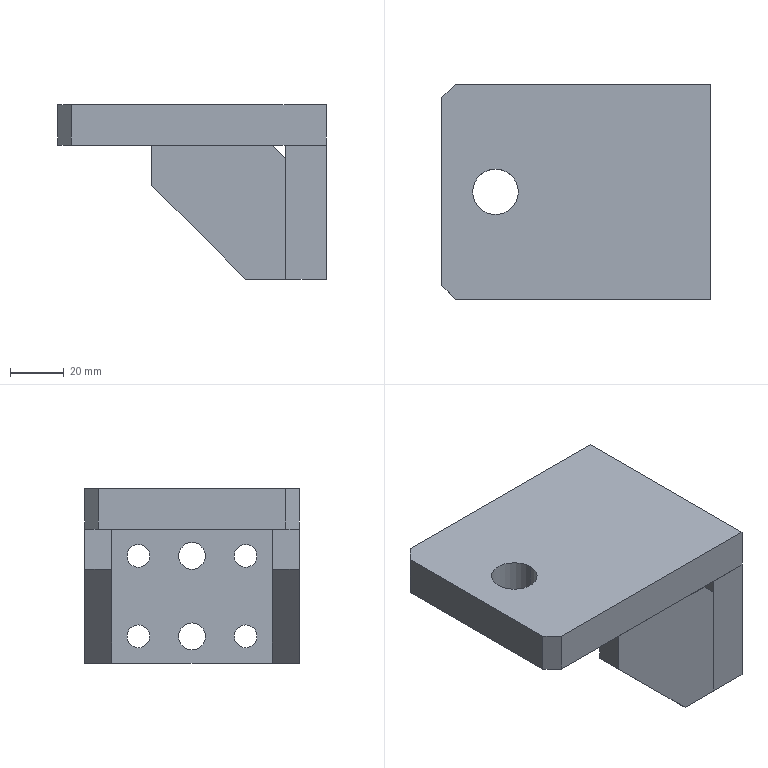Part | SolidWorks | features BaseBody 4 | 4 solids | 44 faces | box 100 x 80 x 65 mm | volume 207959 mm3 | plane 30 | cylinder 14 | commonest cylinder face diameters 8.5 x8 10 x4 17 x2
STEP:
#1=CARTESIAN_POINT('',(35.,40.,-5.));
#2=VERTEX_POINT('',#1);
#3=CARTESIAN_POINT('',(35.,40.,-50.));
#4=VERTEX_POINT('',#3);
#5=CARTESIAN_POINT('',(35.,40.,-5.));
#6=DIRECTION('',(0.,0.,-1.));
#7=VECTOR('',#6,1000.);
#8=LINE('',#5,#7);
#9=EDGE_CURVE('',#2,#4,#8,.T.);
#10=ORIENTED_EDGE('',*,*,#9,.F.);
#11=CARTESIAN_POINT('',(35.,30.,-5.));
#12=VERTEX_POINT('',#11);
#13=CARTESIAN_POINT('',(35.,30.,-5.));
#14=DIRECTION('',(0.,1.,0.));
#15=VECTOR('',#14,1000.);
#16=LINE('',#13,#15);
#17=EDGE_CURVE('',#12,#2,#16,.T.);
#18=ORIENTED_EDGE('',*,*,#17,.F.);
#19=CARTESIAN_POINT('',(35.,30.,-50.));
#20=VERTEX_POINT('',#19);
#21=CARTESIAN_POINT('',(35.,30.,-5.));
#22=DIRECTION('',(0.,0.,-1.));
#23=VECTOR('',#22,1000.);
#24=LINE('',#21,#23);
#25=EDGE_CURVE('',#12,#20,#24,.T.);
#26=ORIENTED_EDGE('',*,*,#25,.T.);
#27=CARTESIAN_POINT('',(35.,30.,-50.));
#28=DIRECTION('',(0.,1.,0.));
#29=VECTOR('',#28,1000.);
#30=LINE('',#27,#29);
#31=EDGE_CURVE('',#20,#4,#30,.T.);
#32=ORIENTED_EDGE('',*,*,#31,.T.);
#33=EDGE_LOOP('',(#10,#18,#26,#32));
#34=FACE_OUTER_BOUND('',#33,.T.);
#35=CARTESIAN_POINT('',(35.,30.,-5.));
#36=DIRECTION('',(1.,0.,0.));
#37=DIRECTION('',(0.,0.,-1.));
#38=AXIS2_PLACEMENT_3D('',#35,#36,#37);
#39=PLANE('',#38);
#40=ADVANCED_FACE('',(#34),#39,.T.);
#41=CARTESIAN_POINT('',(30.,40.,0.));
#42=VERTEX_POINT('',#41);
#43=CARTESIAN_POINT('',(30.,40.,0.));
#44=DIRECTION('',(0.7071,0.,-0.7071));
#45=VECTOR('',#44,1000.);
#46=LINE('',#43,#45);
#47=EDGE_CURVE('',#42,#2,#46,.T.);
#48=ORIENTED_EDGE('',*,*,#47,.F.);
#49=CARTESIAN_POINT('',(30.,30.,0.));
#50=VERTEX_POINT('',#49);
#51=CARTESIAN_POINT('',(30.,30.,0.));
#52=DIRECTION('',(0.,1.,0.));
#53=VECTOR('',#52,1000.);
#54=LINE('',#51,#53);
#55=EDGE_CURVE('',#50,#42,#54,.T.);
#56=ORIENTED_EDGE('',*,*,#55,.F.);
#57=CARTESIAN_POINT('',(30.,30.,0.));
#58=DIRECTION('',(0.7071,0.,-0.7071));
#59=VECTOR('',#58,1000.);
#60=LINE('',#57,#59);
#61=EDGE_CURVE('',#50,#12,#60,.T.);
#62=ORIENTED_EDGE('',*,*,#61,.T.);
#63=ORIENTED_EDGE('',*,*,#17,.T.);
#64=EDGE_LOOP('',(#48,#56,#62,#63));
#65=FACE_OUTER_BOUND('',#64,.T.);
#66=CARTESIAN_POINT('',(30.,30.,0.));
#67=DIRECTION('',(0.7071,0.,0.7071));
#68=DIRECTION('',(0.7071,0.,-0.7071));
#69=AXIS2_PLACEMENT_3D('',#66,#67,#68);
#70=PLANE('',#69);
#71=ADVANCED_FACE('',(#65),#70,.T.);
#72=CARTESIAN_POINT('',(-15.,40.,0.));
#73=VERTEX_POINT('',#72);
#74=CARTESIAN_POINT('',(-15.,40.,0.));
#75=DIRECTION('',(1.,0.,0.));
#76=VECTOR('',#75,1000.);
#77=LINE('',#74,#76);
#78=EDGE_CURVE('',#73,#42,#77,.T.);
#79=ORIENTED_EDGE('',*,*,#78,.F.);
#80=CARTESIAN_POINT('',(-15.,30.,0.));
#81=VERTEX_POINT('',#80);
#82=CARTESIAN_POINT('',(-15.,30.,0.));
#83=DIRECTION('',(0.,1.,0.));
#84=VECTOR('',#83,1000.);
#85=LINE('',#82,#84);
#86=EDGE_CURVE('',#81,#73,#85,.T.);
#87=ORIENTED_EDGE('',*,*,#86,.F.);
#88=CARTESIAN_POINT('',(-15.,30.,0.));
#89=DIRECTION('',(1.,0.,0.));
#90=VECTOR('',#89,1000.);
#91=LINE('',#88,#90);
#92=EDGE_CURVE('',#81,#50,#91,.T.);
#93=ORIENTED_EDGE('',*,*,#92,.T.);
#94=ORIENTED_EDGE('',*,*,#55,.T.);
#95=EDGE_LOOP('',(#79,#87,#93,#94));
#96=FACE_OUTER_BOUND('',#95,.T.);
#97=CARTESIAN_POINT('',(-15.,30.,0.));
#98=DIRECTION('',(0.,0.,1.));
#99=DIRECTION('',(1.,0.,0.));
#100=AXIS2_PLACEMENT_3D('',#97,#98,#99);
#101=PLANE('',#100);
#102=ADVANCED_FACE('',(#96),#101,.T.);
#103=CARTESIAN_POINT('',(-15.,40.,-15.));
#104=VERTEX_POINT('',#103);
#105=CARTESIAN_POINT('',(-15.,40.,-15.));
#106=DIRECTION('',(0.,0.,1.));
#107=VECTOR('',#106,1000.);
#108=LINE('',#105,#107);
#109=EDGE_CURVE('',#104,#73,#108,.T.);
#110=ORIENTED_EDGE('',*,*,#109,.F.);
#111=CARTESIAN_POINT('',(-15.,30.,-15.));
#112=VERTEX_POINT('',#111);
#113=CARTESIAN_POINT('',(-15.,30.,-15.));
#114=DIRECTION('',(0.,1.,0.));
#115=VECTOR('',#114,1000.);
#116=LINE('',#113,#115);
#117=EDGE_CURVE('',#112,#104,#116,.T.);
#118=ORIENTED_EDGE('',*,*,#117,.F.);
#119=CARTESIAN_POINT('',(-15.,30.,-15.));
#120=DIRECTION('',(0.,0.,1.));
#121=VECTOR('',#120,1000.);
#122=LINE('',#119,#121);
#123=EDGE_CURVE('',#112,#81,#122,.T.);
#124=ORIENTED_EDGE('',*,*,#123,.T.);
#125=ORIENTED_EDGE('',*,*,#86,.T.);
#126=EDGE_LOOP('',(#110,#118,#124,#125));
#127=FACE_OUTER_BOUND('',#126,.T.);
#128=CARTESIAN_POINT('',(-15.,30.,-15.));
#129=DIRECTION('',(-1.,0.,0.));
#130=DIRECTION('',(0.,0.,1.));
#131=AXIS2_PLACEMENT_3D('',#128,#129,#130);
#132=PLANE('',#131);
#133=ADVANCED_FACE('',(#127),#132,.T.);
#134=CARTESIAN_POINT('',(20.,40.,-50.));
#135=VERTEX_POINT('',#134);
#136=CARTESIAN_POINT('',(20.,40.,-50.));
#137=DIRECTION('',(-0.7071,0.,0.7071));
#138=VECTOR('',#137,1000.);
#139=LINE('',#136,#138);
#140=EDGE_CURVE('',#135,#104,#139,.T.);
#141=ORIENTED_EDGE('',*,*,#140,.F.);
#142=CARTESIAN_POINT('',(20.,30.,-50.));
#143=VERTEX_POINT('',#142);
#144=CARTESIAN_POINT('',(20.,30.,-50.));
#145=DIRECTION('',(0.,1.,0.));
#146=VECTOR('',#145,1000.);
#147=LINE('',#144,#146);
#148=EDGE_CURVE('',#143,#135,#147,.T.);
#149=ORIENTED_EDGE('',*,*,#148,.F.);
#150=CARTESIAN_POINT('',(20.,30.,-50.));
#151=DIRECTION('',(-0.7071,0.,0.7071));
#152=VECTOR('',#151,1000.);
#153=LINE('',#150,#152);
#154=EDGE_CURVE('',#143,#112,#153,.T.);
#155=ORIENTED_EDGE('',*,*,#154,.T.);
#156=ORIENTED_EDGE('',*,*,#117,.T.);
#157=EDGE_LOOP('',(#141,#149,#155,#156));
#158=FACE_OUTER_BOUND('',#157,.T.);
#159=CARTESIAN_POINT('',(20.,30.,-50.));
#160=DIRECTION('',(-0.7071,0.,-0.7071));
#161=DIRECTION('',(-0.7071,0.,0.7071));
#162=AXIS2_PLACEMENT_3D('',#159,#160,#161);
#163=PLANE('',#162);
#164=ADVANCED_FACE('',(#158),#163,.T.);
#165=CARTESIAN_POINT('',(35.,40.,-50.));
#166=DIRECTION('',(-1.,0.,0.));
#167=VECTOR('',#166,1000.);
#168=LINE('',#165,#167);
#169=EDGE_CURVE('',#4,#135,#168,.T.);
#170=ORIENTED_EDGE('',*,*,#169,.F.);
#171=ORIENTED_EDGE('',*,*,#31,.F.);
#172=CARTESIAN_POINT('',(35.,30.,-50.));
#173=DIRECTION('',(-1.,0.,0.));
#174=VECTOR('',#173,1000.);
#175=LINE('',#172,#174);
#176=EDGE_CURVE('',#20,#143,#175,.T.);
#177=ORIENTED_EDGE('',*,*,#176,.T.);
#178=ORIENTED_EDGE('',*,*,#148,.T.);
#179=EDGE_LOOP('',(#170,#171,#177,#178));
#180=FACE_OUTER_BOUND('',#179,.T.);
#181=CARTESIAN_POINT('',(35.,30.,-50.));
#182=DIRECTION('',(0.,0.,-1.));
#183=DIRECTION('',(-1.,0.,0.));
#184=AXIS2_PLACEMENT_3D('',#181,#182,#183);
#185=PLANE('',#184);
#186=ADVANCED_FACE('',(#180),#185,.T.);
#187=ORIENTED_EDGE('',*,*,#25,.F.);
#188=ORIENTED_EDGE('',*,*,#61,.F.);
#189=ORIENTED_EDGE('',*,*,#92,.F.);
#190=ORIENTED_EDGE('',*,*,#123,.F.);
#191=ORIENTED_EDGE('',*,*,#154,.F.);
#192=ORIENTED_EDGE('',*,*,#176,.F.);
#193=EDGE_LOOP('',(#187,#188,#189,#190,#191,#192));
#194=FACE_OUTER_BOUND('',#193,.T.);
#195=CARTESIAN_POINT('',(0.,30.,0.));
#196=DIRECTION('',(0.,1.,0.));
#197=DIRECTION('',(0.,0.,1.));
#198=AXIS2_PLACEMENT_3D('',#195,#196,#197);
#199=PLANE('',#198);
#200=ADVANCED_FACE('',(#194),#199,.F.);
#201=ORIENTED_EDGE('',*,*,#9,.T.);
#202=ORIENTED_EDGE('',*,*,#169,.T.);
#203=ORIENTED_EDGE('',*,*,#140,.T.);
#204=ORIENTED_EDGE('',*,*,#109,.T.);
#205=ORIENTED_EDGE('',*,*,#78,.T.);
#206=ORIENTED_EDGE('',*,*,#47,.T.);
#207=EDGE_LOOP('',(#201,#202,#203,#204,#205,#206));
#208=FACE_OUTER_BOUND('',#207,.T.);
#209=CARTESIAN_POINT('',(0.,40.,0.));
#210=DIRECTION('',(0.,1.,0.));
#211=DIRECTION('',(0.,0.,1.));
#212=AXIS2_PLACEMENT_3D('',#209,#210,#211);
#213=PLANE('',#212);
#214=ADVANCED_FACE('',(#208),#213,.T.);
#215=CLOSED_SHELL('',(#40,#71,#102,#133,#164,#186,#200,#214));
#216=MANIFOLD_SOLID_BREP('',#215);
#217=CARTESIAN_POINT('',(35.,-30.,-5.));
#218=VERTEX_POINT('',#217);
#219=CARTESIAN_POINT('',(35.,-30.,-50.));
#220=VERTEX_POINT('',#219);
#221=CARTESIAN_POINT('',(35.,-30.,-5.));
#222=DIRECTION('',(0.,0.,-1.));
#223=VECTOR('',#222,1000.);
#224=LINE('',#221,#223);
#225=EDGE_CURVE('',#218,#220,#224,.T.);
#226=ORIENTED_EDGE('',*,*,#225,.F.);
#227=CARTESIAN_POINT('',(35.,-40.,-5.));
#228=VERTEX_POINT('',#227);
#229=CARTESIAN_POINT('',(35.,-40.,-5.));
#230=DIRECTION('',(0.,1.,0.));
#231=VECTOR('',#230,1000.);
#232=LINE('',#229,#231);
#233=EDGE_CURVE('',#228,#218,#232,.T.);
#234=ORIENTED_EDGE('',*,*,#233,.F.);
#235=CARTESIAN_POINT('',(35.,-40.,-50.));
#236=VERTEX_POINT('',#235);
#237=CARTESIAN_POINT('',(35.,-40.,-5.));
#238=DIRECTION('',(0.,0.,-1.));
#239=VECTOR('',#238,1000.);
#240=LINE('',#237,#239);
#241=EDGE_CURVE('',#228,#236,#240,.T.);
#242=ORIENTED_EDGE('',*,*,#241,.T.);
#243=CARTESIAN_POINT('',(35.,-40.,-50.));
#244=DIRECTION('',(0.,1.,0.));
#245=VECTOR('',#244,1000.);
#246=LINE('',#243,#245);
#247=EDGE_CURVE('',#236,#220,#246,.T.);
#248=ORIENTED_EDGE('',*,*,#247,.T.);
#249=EDGE_LOOP('',(#226,#234,#242,#248));
#250=FACE_OUTER_BOUND('',#249,.T.);
#251=CARTESIAN_POINT('',(35.,-40.,-5.));
#252=DIRECTION('',(1.,0.,0.));
#253=DIRECTION('',(0.,0.,-1.));
#254=AXIS2_PLACEMENT_3D('',#251,#252,#253);
#255=PLANE('',#254);
#256=ADVANCED_FACE('',(#250),#255,.T.);
#257=CARTESIAN_POINT('',(30.,-30.,0.));
#258=VERTEX_POINT('',#257);
#259=CARTESIAN_POINT('',(30.,-30.,0.));
#260=DIRECTION('',(0.7071,0.,-0.7071));
#261=VECTOR('',#260,1000.);
#262=LINE('',#259,#261);
#263=EDGE_CURVE('',#258,#218,#262,.T.);
#264=ORIENTED_EDGE('',*,*,#263,.F.);
#265=CARTESIAN_POINT('',(30.,-40.,0.));
#266=VERTEX_POINT('',#265);
#267=CARTESIAN_POINT('',(30.,-40.,0.));
#268=DIRECTION('',(0.,1.,0.));
#269=VECTOR('',#268,1000.);
#270=LINE('',#267,#269);
#271=EDGE_CURVE('',#266,#258,#270,.T.);
#272=ORIENTED_EDGE('',*,*,#271,.F.);
#273=CARTESIAN_POINT('',(30.,-40.,0.));
#274=DIRECTION('',(0.7071,0.,-0.7071));
#275=VECTOR('',#274,1000.);
#276=LINE('',#273,#275);
#277=EDGE_CURVE('',#266,#228,#276,.T.);
#278=ORIENTED_EDGE('',*,*,#277,.T.);
#279=ORIENTED_EDGE('',*,*,#233,.T.);
#280=EDGE_LOOP('',(#264,#272,#278,#279));
#281=FACE_OUTER_BOUND('',#280,.T.);
#282=CARTESIAN_POINT('',(30.,-40.,0.));
#283=DIRECTION('',(0.7071,0.,0.7071));
#284=DIRECTION('',(0.7071,0.,-0.7071));
#285=AXIS2_PLACEMENT_3D('',#282,#283,#284);
#286=PLANE('',#285);
#287=ADVANCED_FACE('',(#281),#286,.T.);
#288=CARTESIAN_POINT('',(-15.,-30.,0.));
#289=VERTEX_POINT('',#288);
#290=CARTESIAN_POINT('',(-15.,-30.,0.));
#291=DIRECTION('',(1.,0.,0.));
#292=VECTOR('',#291,1000.);
#293=LINE('',#290,#292);
#294=EDGE_CURVE('',#289,#258,#293,.T.);
#295=ORIENTED_EDGE('',*,*,#294,.F.);
#296=CARTESIAN_POINT('',(-15.,-40.,0.));
#297=VERTEX_POINT('',#296);
#298=CARTESIAN_POINT('',(-15.,-40.,0.));
#299=DIRECTION('',(0.,1.,0.));
#300=VECTOR('',#299,1000.);
#301=LINE('',#298,#300);
#302=EDGE_CURVE('',#297,#289,#301,.T.);
#303=ORIENTED_EDGE('',*,*,#302,.F.);
#304=CARTESIAN_POINT('',(-15.,-40.,0.));
#305=DIRECTION('',(1.,0.,0.));
#306=VECTOR('',#305,1000.);
#307=LINE('',#304,#306);
#308=EDGE_CURVE('',#297,#266,#307,.T.);
#309=ORIENTED_EDGE('',*,*,#308,.T.);
#310=ORIENTED_EDGE('',*,*,#271,.T.);
#311=EDGE_LOOP('',(#295,#303,#309,#310));
#312=FACE_OUTER_BOUND('',#311,.T.);
#313=CARTESIAN_POINT('',(-15.,-40.,0.));
#314=DIRECTION('',(0.,0.,1.));
#315=DIRECTION('',(1.,0.,0.));
#316=AXIS2_PLACEMENT_3D('',#313,#314,#315);
#317=PLANE('',#316);
#318=ADVANCED_FACE('',(#312),#317,.T.);
#319=CARTESIAN_POINT('',(-15.,-30.,-15.));
#320=VERTEX_POINT('',#319);
#321=CARTESIAN_POINT('',(-15.,-30.,-15.));
#322=DIRECTION('',(0.,0.,1.));
#323=VECTOR('',#322,1000.);
#324=LINE('',#321,#323);
#325=EDGE_CURVE('',#320,#289,#324,.T.);
#326=ORIENTED_EDGE('',*,*,#325,.F.);
#327=CARTESIAN_POINT('',(-15.,-40.,-15.));
#328=VERTEX_POINT('',#327);
#329=CARTESIAN_POINT('',(-15.,-40.,-15.));
#330=DIRECTION('',(0.,1.,0.));
#331=VECTOR('',#330,1000.);
#332=LINE('',#329,#331);
#333=EDGE_CURVE('',#328,#320,#332,.T.);
#334=ORIENTED_EDGE('',*,*,#333,.F.);
#335=CARTESIAN_POINT('',(-15.,-40.,-15.));
#336=DIRECTION('',(0.,0.,1.));
#337=VECTOR('',#336,1000.);
#338=LINE('',#335,#337);
#339=EDGE_CURVE('',#328,#297,#338,.T.);
#340=ORIENTED_EDGE('',*,*,#339,.T.);
#341=ORIENTED_EDGE('',*,*,#302,.T.);
#342=EDGE_LOOP('',(#326,#334,#340,#341));
#343=FACE_OUTER_BOUND('',#342,.T.);
#344=CARTESIAN_POINT('',(-15.,-40.,-15.));
#345=DIRECTION('',(-1.,0.,0.));
#346=DIRECTION('',(0.,0.,1.));
#347=AXIS2_PLACEMENT_3D('',#344,#345,#346);
#348=PLANE('',#347);
#349=ADVANCED_FACE('',(#343),#348,.T.);
#350=CARTESIAN_POINT('',(20.,-30.,-50.));
#351=VERTEX_POINT('',#350);
#352=CARTESIAN_POINT('',(20.,-30.,-50.));
#353=DIRECTION('',(-0.7071,0.,0.7071));
#354=VECTOR('',#353,1000.);
#355=LINE('',#352,#354);
#356=EDGE_CURVE('',#351,#320,#355,.T.);
#357=ORIENTED_EDGE('',*,*,#356,.F.);
#358=CARTESIAN_POINT('',(20.,-40.,-50.));
#359=VERTEX_POINT('',#358);
#360=CARTESIAN_POINT('',(20.,-40.,-50.));
#361=DIRECTION('',(0.,1.,0.));
#362=VECTOR('',#361,1000.);
#363=LINE('',#360,#362);
#364=EDGE_CURVE('',#359,#351,#363,.T.);
#365=ORIENTED_EDGE('',*,*,#364,.F.);
#366=CARTESIAN_POINT('',(20.,-40.,-50.));
#367=DIRECTION('',(-0.7071,0.,0.7071));
#368=VECTOR('',#367,1000.);
#369=LINE('',#366,#368);
#370=EDGE_CURVE('',#359,#328,#369,.T.);
#371=ORIENTED_EDGE('',*,*,#370,.T.);
#372=ORIENTED_EDGE('',*,*,#333,.T.);
#373=EDGE_LOOP('',(#357,#365,#371,#372));
#374=FACE_OUTER_BOUND('',#373,.T.);
#375=CARTESIAN_POINT('',(20.,-40.,-50.));
#376=DIRECTION('',(-0.7071,0.,-0.7071));
#377=DIRECTION('',(-0.7071,0.,0.7071));
#378=AXIS2_PLACEMENT_3D('',#375,#376,#377);
#379=PLANE('',#378);
#380=ADVANCED_FACE('',(#374),#379,.T.);
#381=CARTESIAN_POINT('',(35.,-30.,-50.));
#382=DIRECTION('',(-1.,0.,0.));
#383=VECTOR('',#382,1000.);
#384=LINE('',#381,#383);
#385=EDGE_CURVE('',#220,#351,#384,.T.);
#386=ORIENTED_EDGE('',*,*,#385,.F.);
#387=ORIENTED_EDGE('',*,*,#247,.F.);
#388=CARTESIAN_POINT('',(35.,-40.,-50.));
#389=DIRECTION('',(-1.,0.,0.));
#390=VECTOR('',#389,1000.);
#391=LINE('',#388,#390);
#392=EDGE_CURVE('',#236,#359,#391,.T.);
#393=ORIENTED_EDGE('',*,*,#392,.T.);
#394=ORIENTED_EDGE('',*,*,#364,.T.);
#395=EDGE_LOOP('',(#386,#387,#393,#394));
#396=FACE_OUTER_BOUND('',#395,.T.);
#397=CARTESIAN_POINT('',(35.,-40.,-50.));
#398=DIRECTION('',(0.,0.,-1.));
#399=DIRECTION('',(-1.,0.,0.));
#400=AXIS2_PLACEMENT_3D('',#397,#398,#399);
#401=PLANE('',#400);
#402=ADVANCED_FACE('',(#396),#401,.T.);
#403=ORIENTED_EDGE('',*,*,#241,.F.);
#404=ORIENTED_EDGE('',*,*,#277,.F.);
#405=ORIENTED_EDGE('',*,*,#308,.F.);
#406=ORIENTED_EDGE('',*,*,#339,.F.);
#407=ORIENTED_EDGE('',*,*,#370,.F.);
#408=ORIENTED_EDGE('',*,*,#392,.F.);
#409=EDGE_LOOP('',(#403,#404,#405,#406,#407,#408));
#410=FACE_OUTER_BOUND('',#409,.T.);
#411=CARTESIAN_POINT('',(0.,-40.,0.));
#412=DIRECTION('',(0.,1.,0.));
#413=DIRECTION('',(0.,0.,1.));
#414=AXIS2_PLACEMENT_3D('',#411,#412,#413);
#415=PLANE('',#414);
#416=ADVANCED_FACE('',(#410),#415,.F.);
#417=ORIENTED_EDGE('',*,*,#225,.T.);
#418=ORIENTED_EDGE('',*,*,#385,.T.);
#419=ORIENTED_EDGE('',*,*,#356,.T.);
#420=ORIENTED_EDGE('',*,*,#325,.T.);
#421=ORIENTED_EDGE('',*,*,#294,.T.);
#422=ORIENTED_EDGE('',*,*,#263,.T.);
#423=EDGE_LOOP('',(#417,#418,#419,#420,#421,#422));
#424=FACE_OUTER_BOUND('',#423,.T.);
#425=CARTESIAN_POINT('',(0.,-30.,0.));
#426=DIRECTION('',(0.,1.,0.));
#427=DIRECTION('',(0.,0.,1.));
#428=AXIS2_PLACEMENT_3D('',#425,#426,#427);
#429=PLANE('',#428);
#430=ADVANCED_FACE('',(#424),#429,.T.);
#431=CLOSED_SHELL('',(#256,#287,#318,#349,#380,#402,#416,#430));
#432=MANIFOLD_SOLID_BREP('',#431);
#433=CARTESIAN_POINT('',(-38.5,0.,0.));
#434=VERTEX_POINT('',#433);
#435=CARTESIAN_POINT('',(-21.5,0.,0.));
#436=VERTEX_POINT('',#435);
#437=CARTESIAN_POINT('',(-30.,0.,0.));
#438=DIRECTION('',(0.,0.,1.));
#439=DIRECTION('',(1.,0.,0.));
#440=AXIS2_PLACEMENT_3D('',#437,#438,#439);
#441=CIRCLE('',#440,8.5);
#442=EDGE_CURVE('',#434,#436,#441,.T.);
#443=ORIENTED_EDGE('',*,*,#442,.F.);
#444=CARTESIAN_POINT('',(-38.5,0.,15.));
#445=VERTEX_POINT('',#444);
#446=CARTESIAN_POINT('',(-38.5,0.,15.));
#447=DIRECTION('',(0.,0.,1.));
#448=VECTOR('',#447,1000.);
#449=LINE('',#446,#448);
#450=EDGE_CURVE('',#434,#445,#449,.T.);
#451=ORIENTED_EDGE('',*,*,#450,.T.);
#452=CARTESIAN_POINT('',(-21.5,0.,15.));
#453=VERTEX_POINT('',#452);
#454=CARTESIAN_POINT('',(-30.,0.,15.));
#455=DIRECTION('',(0.,0.,1.));
#456=DIRECTION('',(1.,0.,0.));
#457=AXIS2_PLACEMENT_3D('',#454,#455,#456);
#458=CIRCLE('',#457,8.5);
#459=EDGE_CURVE('',#445,#453,#458,.T.);
#460=ORIENTED_EDGE('',*,*,#459,.T.);
#461=CARTESIAN_POINT('',(-21.5,0.,15.));
#462=DIRECTION('',(0.,0.,1.));
#463=VECTOR('',#462,1000.);
#464=LINE('',#461,#463);
#465=EDGE_CURVE('',#436,#453,#464,.T.);
#466=ORIENTED_EDGE('',*,*,#465,.F.);
#467=EDGE_LOOP('',(#443,#451,#460,#466));
#468=FACE_OUTER_BOUND('',#467,.T.);
#469=CARTESIAN_POINT('',(-30.,0.,15.));
#470=DIRECTION('',(0.,0.,1.));
#471=DIRECTION('',(1.,0.,0.));
#472=AXIS2_PLACEMENT_3D('',#469,#470,#471);
#473=CYLINDRICAL_SURFACE('',#472,8.5);
#474=ADVANCED_FACE('',(#468),#473,.F.);
#475=CARTESIAN_POINT('',(50.,-40.,0.));
#476=VERTEX_POINT('',#475);
#477=CARTESIAN_POINT('',(50.,40.,0.));
#478=VERTEX_POINT('',#477);
#479=CARTESIAN_POINT('',(50.,40.,0.));
#480=DIRECTION('',(0.,1.,0.));
#481=VECTOR('',#480,1000.);
#482=LINE('',#479,#481);
#483=EDGE_CURVE('',#476,#478,#482,.T.);
#484=ORIENTED_EDGE('',*,*,#483,.T.);
#485=CARTESIAN_POINT('',(50.,40.,15.));
#486=VERTEX_POINT('',#485);
#487=CARTESIAN_POINT('',(50.,40.,15.));
#488=DIRECTION('',(0.,0.,-1.));
#489=VECTOR('',#488,1000.);
#490=LINE('',#487,#489);
#491=EDGE_CURVE('',#486,#478,#490,.T.);
#492=ORIENTED_EDGE('',*,*,#491,.F.);
#493=CARTESIAN_POINT('',(50.,-40.,15.));
#494=VERTEX_POINT('',#493);
#495=CARTESIAN_POINT('',(50.,40.,15.));
#496=DIRECTION('',(0.,1.,0.));
#497=VECTOR('',#496,1000.);
#498=LINE('',#495,#497);
#499=EDGE_CURVE('',#494,#486,#498,.T.);
#500=ORIENTED_EDGE('',*,*,#499,.F.);
#501=CARTESIAN_POINT('',(50.,-40.,15.));
#502=DIRECTION('',(0.,0.,-1.));
#503=VECTOR('',#502,1000.);
#504=LINE('',#501,#503);
#505=EDGE_CURVE('',#494,#476,#504,.T.);
#506=ORIENTED_EDGE('',*,*,#505,.T.);
#507=EDGE_LOOP('',(#484,#492,#500,#506));
#508=FACE_OUTER_BOUND('',#507,.T.);
#509=CARTESIAN_POINT('',(50.,40.,15.));
#510=DIRECTION('',(-1.,0.,0.));
#511=DIRECTION('',(0.,-1.,0.));
#512=AXIS2_PLACEMENT_3D('',#509,#510,#511);
#513=PLANE('',#512);
#514=ADVANCED_FACE('',(#508),#513,.F.);
#515=CARTESIAN_POINT('',(-45.,40.,0.));
#516=VERTEX_POINT('',#515);
#517=CARTESIAN_POINT('',(-50.,40.,0.));
#518=DIRECTION('',(-1.,0.,0.));
#519=VECTOR('',#518,1000.);
#520=LINE('',#517,#519);
#521=EDGE_CURVE('',#478,#516,#520,.T.);
#522=ORIENTED_EDGE('',*,*,#521,.T.);
#523=CARTESIAN_POINT('',(-45.,40.,15.));
#524=VERTEX_POINT('',#523);
#525=CARTESIAN_POINT('',(-45.,40.,15.));
#526=DIRECTION('',(0.,0.,1.));
#527=VECTOR('',#526,1000.);
#528=LINE('',#525,#527);
#529=EDGE_CURVE('',#516,#524,#528,.T.);
#530=ORIENTED_EDGE('',*,*,#529,.T.);
#531=CARTESIAN_POINT('',(-50.,40.,15.));
#532=DIRECTION('',(-1.,0.,0.));
#533=VECTOR('',#532,1000.);
#534=LINE('',#531,#533);
#535=EDGE_CURVE('',#486,#524,#534,.T.);
#536=ORIENTED_EDGE('',*,*,#535,.F.);
#537=ORIENTED_EDGE('',*,*,#491,.T.);
#538=EDGE_LOOP('',(#522,#530,#536,#537));
#539=FACE_OUTER_BOUND('',#538,.T.);
#540=CARTESIAN_POINT('',(-50.,40.,15.));
#541=DIRECTION('',(0.,-1.,0.));
#542=DIRECTION('',(0.,0.,-1.));
#543=AXIS2_PLACEMENT_3D('',#540,#541,#542);
#544=PLANE('',#543);
#545=ADVANCED_FACE('',(#539),#544,.F.);
#546=CARTESIAN_POINT('',(-50.,35.,0.));
#547=VERTEX_POINT('',#546);
#548=CARTESIAN_POINT('',(-50.,-35.,0.));
#549=VERTEX_POINT('',#548);
#550=CARTESIAN_POINT('',(-50.,40.,0.));
#551=DIRECTION('',(0.,-1.,0.));
#552=VECTOR('',#551,1000.);
#553=LINE('',#550,#552);
#554=EDGE_CURVE('',#547,#549,#553,.T.);
#555=ORIENTED_EDGE('',*,*,#554,.T.);
#556=CARTESIAN_POINT('',(-50.,-35.,15.));
#557=VERTEX_POINT('',#556);
#558=CARTESIAN_POINT('',(-50.,-35.,15.));
#559=DIRECTION('',(0.,0.,1.));
#560=VECTOR('',#559,1000.);
#561=LINE('',#558,#560);
#562=EDGE_CURVE('',#549,#557,#561,.T.);
#563=ORIENTED_EDGE('',*,*,#562,.T.);
#564=CARTESIAN_POINT('',(-50.,35.,15.));
#565=VERTEX_POINT('',#564);
#566=CARTESIAN_POINT('',(-50.,40.,15.));
#567=DIRECTION('',(0.,-1.,0.));
#568=VECTOR('',#567,1000.);
#569=LINE('',#566,#568);
#570=EDGE_CURVE('',#565,#557,#569,.T.);
#571=ORIENTED_EDGE('',*,*,#570,.F.);
#572=CARTESIAN_POINT('',(-50.,35.,15.));
#573=DIRECTION('',(0.,0.,-1.));
#574=VECTOR('',#573,1000.);
#575=LINE('',#572,#574);
#576=EDGE_CURVE('',#565,#547,#575,.T.);
#577=ORIENTED_EDGE('',*,*,#576,.T.);
#578=EDGE_LOOP('',(#555,#563,#571,#577));
#579=FACE_OUTER_BOUND('',#578,.T.);
#580=CARTESIAN_POINT('',(-50.,40.,15.));
#581=DIRECTION('',(1.,0.,0.));
#582=DIRECTION('',(0.,1.,0.));
#583=AXIS2_PLACEMENT_3D('',#580,#581,#582);
#584=PLANE('',#583);
#585=ADVANCED_FACE('',(#579),#584,.F.);
#586=CARTESIAN_POINT('',(-45.,-40.,15.));
#587=VERTEX_POINT('',#586);
#588=CARTESIAN_POINT('',(-50.,-40.,15.));
#589=DIRECTION('',(1.,0.,0.));
#590=VECTOR('',#589,1000.);
#591=LINE('',#588,#590);
#592=EDGE_CURVE('',#587,#494,#591,.T.);
#593=ORIENTED_EDGE('',*,*,#592,.F.);
#594=CARTESIAN_POINT('',(-45.,-40.,0.));
#595=VERTEX_POINT('',#594);
#596=CARTESIAN_POINT('',(-45.,-40.,15.));
#597=DIRECTION('',(0.,0.,-1.));
#598=VECTOR('',#597,1000.);
#599=LINE('',#596,#598);
#600=EDGE_CURVE('',#587,#595,#599,.T.);
#601=ORIENTED_EDGE('',*,*,#600,.T.);
#602=CARTESIAN_POINT('',(-50.,-40.,0.));
#603=DIRECTION('',(1.,0.,0.));
#604=VECTOR('',#603,1000.);
#605=LINE('',#602,#604);
#606=EDGE_CURVE('',#595,#476,#605,.T.);
#607=ORIENTED_EDGE('',*,*,#606,.T.);
#608=ORIENTED_EDGE('',*,*,#505,.F.);
#609=EDGE_LOOP('',(#593,#601,#607,#608));
#610=FACE_OUTER_BOUND('',#609,.T.);
#611=CARTESIAN_POINT('',(-50.,-40.,15.));
#612=DIRECTION('',(0.,1.,0.));
#613=DIRECTION('',(0.,0.,1.));
#614=AXIS2_PLACEMENT_3D('',#611,#612,#613);
#615=PLANE('',#614);
#616=ADVANCED_FACE('',(#610),#615,.F.);
#617=CARTESIAN_POINT('',(-30.,0.,15.));
#618=DIRECTION('',(0.,0.,1.));
#619=DIRECTION('',(1.,0.,0.));
#620=AXIS2_PLACEMENT_3D('',#617,#618,#619);
#621=CIRCLE('',#620,8.5);
#622=EDGE_CURVE('',#453,#445,#621,.T.);
#623=ORIENTED_EDGE('',*,*,#622,.F.);
#624=ORIENTED_EDGE('',*,*,#459,.F.);
#625=EDGE_LOOP('',(#623,#624));
#626=FACE_BOUND('',#625,.T.);
#627=ORIENTED_EDGE('',*,*,#570,.T.);
#628=CARTESIAN_POINT('',(-42.5,-42.5,15.));
#629=DIRECTION('',(0.7071,-0.7071,0.));
#630=VECTOR('',#629,1000.);
#631=LINE('',#628,#630);
#632=EDGE_CURVE('',#557,#587,#631,.T.);
#633=ORIENTED_EDGE('',*,*,#632,.T.);
#634=ORIENTED_EDGE('',*,*,#592,.T.);
#635=ORIENTED_EDGE('',*,*,#499,.T.);
#636=ORIENTED_EDGE('',*,*,#535,.T.);
#637=CARTESIAN_POINT('',(-42.5,42.5,15.));
#638=DIRECTION('',(-0.7071,-0.7071,0.));
#639=VECTOR('',#638,1000.);
#640=LINE('',#637,#639);
#641=EDGE_CURVE('',#524,#565,#640,.T.);
#642=ORIENTED_EDGE('',*,*,#641,.T.);
#643=EDGE_LOOP('',(#627,#633,#634,#635,#636,#642));
#644=FACE_OUTER_BOUND('',#643,.T.);
#645=CARTESIAN_POINT('',(0.,0.,15.));
#646=DIRECTION('',(0.,0.,1.));
#647=DIRECTION('',(1.,0.,0.));
#648=AXIS2_PLACEMENT_3D('',#645,#646,#647);
#649=PLANE('',#648);
#650=ADVANCED_FACE('',(#626,#644),#649,.T.);
#651=CARTESIAN_POINT('',(-30.,0.,0.));
#652=DIRECTION('',(0.,0.,1.));
#653=DIRECTION('',(1.,0.,0.));
#654=AXIS2_PLACEMENT_3D('',#651,#652,#653);
#655=CIRCLE('',#654,8.5);
#656=EDGE_CURVE('',#436,#434,#655,.T.);
#657=ORIENTED_EDGE('',*,*,#656,.T.);
#658=ORIENTED_EDGE('',*,*,#442,.T.);
#659=EDGE_LOOP('',(#657,#658));
#660=FACE_BOUND('',#659,.T.);
#661=ORIENTED_EDGE('',*,*,#606,.F.);
#662=CARTESIAN_POINT('',(-45.,-40.,0.));
#663=DIRECTION('',(-0.7071,0.7071,0.));
#664=VECTOR('',#663,1000.);
#665=LINE('',#662,#664);
#666=EDGE_CURVE('',#595,#549,#665,.T.);
#667=ORIENTED_EDGE('',*,*,#666,.T.);
#668=ORIENTED_EDGE('',*,*,#554,.F.);
#669=CARTESIAN_POINT('',(-50.,35.,0.));
#670=DIRECTION('',(0.7071,0.7071,0.));
#671=VECTOR('',#670,1000.);
#672=LINE('',#669,#671);
#673=EDGE_CURVE('',#547,#516,#672,.T.);
#674=ORIENTED_EDGE('',*,*,#673,.T.);
#675=ORIENTED_EDGE('',*,*,#521,.F.);
#676=ORIENTED_EDGE('',*,*,#483,.F.);
#677=EDGE_LOOP('',(#661,#667,#668,#674,#675,#676));
#678=FACE_OUTER_BOUND('',#677,.T.);
#679=CARTESIAN_POINT('',(0.,0.,0.));
#680=DIRECTION('',(0.,0.,1.));
#681=DIRECTION('',(1.,0.,0.));
#682=AXIS2_PLACEMENT_3D('',#679,#680,#681);
#683=PLANE('',#682);
#684=ADVANCED_FACE('',(#660,#678),#683,.F.);
#685=ORIENTED_EDGE('',*,*,#450,.F.);
#686=ORIENTED_EDGE('',*,*,#656,.F.);
#687=ORIENTED_EDGE('',*,*,#465,.T.);
#688=ORIENTED_EDGE('',*,*,#622,.T.);
#689=EDGE_LOOP('',(#685,#686,#687,#688));
#690=FACE_OUTER_BOUND('',#689,.T.);
#691=CARTESIAN_POINT('',(-30.,0.,15.));
#692=DIRECTION('',(0.,0.,1.));
#693=DIRECTION('',(1.,0.,0.));
#694=AXIS2_PLACEMENT_3D('',#691,#692,#693);
#695=CYLINDRICAL_SURFACE('',#694,8.5);
#696=ADVANCED_FACE('',(#690),#695,.F.);
#697=ORIENTED_EDGE('',*,*,#632,.F.);
#698=ORIENTED_EDGE('',*,*,#562,.F.);
#699=ORIENTED_EDGE('',*,*,#666,.F.);
#700=ORIENTED_EDGE('',*,*,#600,.F.);
#701=EDGE_LOOP('',(#697,#698,#699,#700));
#702=FACE_OUTER_BOUND('',#701,.T.);
#703=CARTESIAN_POINT('',(-45.,-40.,15.));
#704=DIRECTION('',(0.7071,0.7071,0.));
#705=DIRECTION('',(0.,0.,-1.));
#706=AXIS2_PLACEMENT_3D('',#703,#704,#705);
#707=PLANE('',#706);
#708=ADVANCED_FACE('',(#702),#707,.F.);
#709=ORIENTED_EDGE('',*,*,#641,.F.);
#710=ORIENTED_EDGE('',*,*,#529,.F.);
#711=ORIENTED_EDGE('',*,*,#673,.F.);
#712=ORIENTED_EDGE('',*,*,#576,.F.);
#713=EDGE_LOOP('',(#709,#710,#711,#712));
#714=FACE_OUTER_BOUND('',#713,.T.);
#715=CARTESIAN_POINT('',(-50.,35.,15.));
#716=DIRECTION('',(0.7071,-0.7071,0.));
#717=DIRECTION('',(0.,0.,-1.));
#718=AXIS2_PLACEMENT_3D('',#715,#716,#717);
#719=PLANE('',#718);
#720=ADVANCED_FACE('',(#714),#719,.F.);
#721=CLOSED_SHELL('',(#474,#514,#545,#585,#616,#650,#684,#696,#708,#720));
#722=MANIFOLD_SOLID_BREP('',#721);
#723=CARTESIAN_POINT('',(35.,0.,-5.));
#724=VERTEX_POINT('',#723);
#725=CARTESIAN_POINT('',(35.,0.,-15.));
#726=VERTEX_POINT('',#725);
#727=CARTESIAN_POINT('',(35.,0.,-10.));
#728=DIRECTION('',(1.,0.,0.));
#729=DIRECTION('',(0.,1.,0.));
#730=AXIS2_PLACEMENT_3D('',#727,#728,#729);
#731=CIRCLE('',#730,5.);
#732=EDGE_CURVE('',#724,#726,#731,.T.);
#733=ORIENTED_EDGE('',*,*,#732,.F.);
#734=CARTESIAN_POINT('',(50.,0.,-5.));
#735=VERTEX_POINT('',#734);
#736=CARTESIAN_POINT('',(50.,0.,-5.));
#737=DIRECTION('',(1.,0.,0.));
#738=VECTOR('',#737,1000.);
#739=LINE('',#736,#738);
#740=EDGE_CURVE('',#724,#735,#739,.T.);
#741=ORIENTED_EDGE('',*,*,#740,.T.);
#742=CARTESIAN_POINT('',(50.,0.,-15.));
#743=VERTEX_POINT('',#742);
#744=CARTESIAN_POINT('',(50.,0.,-10.));
#745=DIRECTION('',(1.,0.,0.));
#746=DIRECTION('',(0.,0.,-1.));
#747=AXIS2_PLACEMENT_3D('',#744,#745,#746);
#748=CIRCLE('',#747,5.);
#749=EDGE_CURVE('',#735,#743,#748,.T.);
#750=ORIENTED_EDGE('',*,*,#749,.T.);
#751=CARTESIAN_POINT('',(50.,0.,-15.));
#752=DIRECTION('',(1.,0.,0.));
#753=VECTOR('',#752,1000.);
#754=LINE('',#751,#753);
#755=EDGE_CURVE('',#726,#743,#754,.T.);
#756=ORIENTED_EDGE('',*,*,#755,.F.);
#757=EDGE_LOOP('',(#733,#741,#750,#756));
#758=FACE_OUTER_BOUND('',#757,.T.);
#759=CARTESIAN_POINT('',(50.,0.,-10.));
#760=DIRECTION('',(1.,0.,0.));
#761=DIRECTION('',(0.,0.,-1.));
#762=AXIS2_PLACEMENT_3D('',#759,#760,#761);
#763=CYLINDRICAL_SURFACE('',#762,5.);
#764=ADVANCED_FACE('',(#758),#763,.F.);
#765=CARTESIAN_POINT('',(35.,0.,-35.));
#766=VERTEX_POINT('',#765);
#767=CARTESIAN_POINT('',(35.,0.,-45.));
#768=VERTEX_POINT('',#767);
#769=CARTESIAN_POINT('',(35.,0.,-40.));
#770=DIRECTION('',(1.,0.,0.));
#771=DIRECTION('',(0.,1.,0.));
#772=AXIS2_PLACEMENT_3D('',#769,#770,#771);
#773=CIRCLE('',#772,5.);
#774=EDGE_CURVE('',#766,#768,#773,.T.);
#775=ORIENTED_EDGE('',*,*,#774,.F.);
#776=CARTESIAN_POINT('',(50.,0.,-35.));
#777=VERTEX_POINT('',#776);
#778=CARTESIAN_POINT('',(50.,0.,-35.));
#779=DIRECTION('',(1.,0.,0.));
#780=VECTOR('',#779,1000.);
#781=LINE('',#778,#780);
#782=EDGE_CURVE('',#766,#777,#781,.T.);
#783=ORIENTED_EDGE('',*,*,#782,.T.);
#784=CARTESIAN_POINT('',(50.,0.,-45.));
#785=VERTEX_POINT('',#784);
#786=CARTESIAN_POINT('',(50.,0.,-40.));
#787=DIRECTION('',(1.,0.,0.));
#788=DIRECTION('',(0.,0.,-1.));
#789=AXIS2_PLACEMENT_3D('',#786,#787,#788);
#790=CIRCLE('',#789,5.);
#791=EDGE_CURVE('',#777,#785,#790,.T.);
#792=ORIENTED_EDGE('',*,*,#791,.T.);
#793=CARTESIAN_POINT('',(50.,0.,-45.));
#794=DIRECTION('',(1.,0.,0.));
#795=VECTOR('',#794,1000.);
#796=LINE('',#793,#795);
#797=EDGE_CURVE('',#768,#785,#796,.T.);
#798=ORIENTED_EDGE('',*,*,#797,.F.);
#799=EDGE_LOOP('',(#775,#783,#792,#798));
#800=FACE_OUTER_BOUND('',#799,.T.);
#801=CARTESIAN_POINT('',(50.,0.,-40.));
#802=DIRECTION('',(1.,0.,0.));
#803=DIRECTION('',(0.,0.,-1.));
#804=AXIS2_PLACEMENT_3D('',#801,#802,#803);
#805=CYLINDRICAL_SURFACE('',#804,5.);
#806=ADVANCED_FACE('',(#800),#805,.F.);
#807=CARTESIAN_POINT('',(35.,20.,-5.75));
#808=VERTEX_POINT('',#807);
#809=CARTESIAN_POINT('',(35.,20.,-14.25));
#810=VERTEX_POINT('',#809);
#811=CARTESIAN_POINT('',(35.,20.,-10.));
#812=DIRECTION('',(1.,0.,0.));
#813=DIRECTION('',(0.,1.,0.));
#814=AXIS2_PLACEMENT_3D('',#811,#812,#813);
#815=CIRCLE('',#814,4.25);
#816=EDGE_CURVE('',#808,#810,#815,.T.);
#817=ORIENTED_EDGE('',*,*,#816,.F.);
#818=CARTESIAN_POINT('',(50.,20.,-5.75));
#819=VERTEX_POINT('',#818);
#820=CARTESIAN_POINT('',(50.,20.,-5.75));
#821=DIRECTION('',(1.,0.,0.));
#822=VECTOR('',#821,1000.);
#823=LINE('',#820,#822);
#824=EDGE_CURVE('',#808,#819,#823,.T.);
#825=ORIENTED_EDGE('',*,*,#824,.T.);
#826=CARTESIAN_POINT('',(50.,20.,-14.25));
#827=VERTEX_POINT('',#826);
#828=CARTESIAN_POINT('',(50.,20.,-10.));
#829=DIRECTION('',(1.,0.,0.));
#830=DIRECTION('',(0.,0.,-1.));
#831=AXIS2_PLACEMENT_3D('',#828,#829,#830);
#832=CIRCLE('',#831,4.25);
#833=EDGE_CURVE('',#819,#827,#832,.T.);
#834=ORIENTED_EDGE('',*,*,#833,.T.);
#835=CARTESIAN_POINT('',(50.,20.,-14.25));
#836=DIRECTION('',(1.,0.,0.));
#837=VECTOR('',#836,1000.);
#838=LINE('',#835,#837);
#839=EDGE_CURVE('',#810,#827,#838,.T.);
#840=ORIENTED_EDGE('',*,*,#839,.F.);
#841=EDGE_LOOP('',(#817,#825,#834,#840));
#842=FACE_OUTER_BOUND('',#841,.T.);
#843=CARTESIAN_POINT('',(50.,20.,-10.));
#844=DIRECTION('',(1.,0.,0.));
#845=DIRECTION('',(0.,0.,-1.));
#846=AXIS2_PLACEMENT_3D('',#843,#844,#845);
#847=CYLINDRICAL_SURFACE('',#846,4.25);
#848=ADVANCED_FACE('',(#842),#847,.F.);
#849=CARTESIAN_POINT('',(35.,20.,-35.75));
#850=VERTEX_POINT('',#849);
#851=CARTESIAN_POINT('',(35.,20.,-44.25));
#852=VERTEX_POINT('',#851);
#853=CARTESIAN_POINT('',(35.,20.,-40.));
#854=DIRECTION('',(1.,0.,0.));
#855=DIRECTION('',(0.,1.,0.));
#856=AXIS2_PLACEMENT_3D('',#853,#854,#855);
#857=CIRCLE('',#856,4.25);
#858=EDGE_CURVE('',#850,#852,#857,.T.);
#859=ORIENTED_EDGE('',*,*,#858,.F.);
#860=CARTESIAN_POINT('',(50.,20.,-35.75));
#861=VERTEX_POINT('',#860);
#862=CARTESIAN_POINT('',(50.,20.,-35.75));
#863=DIRECTION('',(1.,0.,0.));
#864=VECTOR('',#863,1000.);
#865=LINE('',#862,#864);
#866=EDGE_CURVE('',#850,#861,#865,.T.);
#867=ORIENTED_EDGE('',*,*,#866,.T.);
#868=CARTESIAN_POINT('',(50.,20.,-44.25));
#869=VERTEX_POINT('',#868);
#870=CARTESIAN_POINT('',(50.,20.,-40.));
#871=DIRECTION('',(1.,0.,0.));
#872=DIRECTION('',(0.,0.,-1.));
#873=AXIS2_PLACEMENT_3D('',#870,#871,#872);
#874=CIRCLE('',#873,4.25);
#875=EDGE_CURVE('',#861,#869,#874,.T.);
#876=ORIENTED_EDGE('',*,*,#875,.T.);
#877=CARTESIAN_POINT('',(50.,20.,-44.25));
#878=DIRECTION('',(1.,0.,0.));
#879=VECTOR('',#878,1000.);
#880=LINE('',#877,#879);
#881=EDGE_CURVE('',#852,#869,#880,.T.);
#882=ORIENTED_EDGE('',*,*,#881,.F.);
#883=EDGE_LOOP('',(#859,#867,#876,#882));
#884=FACE_OUTER_BOUND('',#883,.T.);
#885=CARTESIAN_POINT('',(50.,20.,-40.));
#886=DIRECTION('',(1.,0.,0.));
#887=DIRECTION('',(0.,0.,-1.));
#888=AXIS2_PLACEMENT_3D('',#885,#886,#887);
#889=CYLINDRICAL_SURFACE('',#888,4.25);
#890=ADVANCED_FACE('',(#884),#889,.F.);
#891=CARTESIAN_POINT('',(35.,-20.,-35.75));
#892=VERTEX_POINT('',#891);
#893=CARTESIAN_POINT('',(35.,-20.,-44.25));
#894=VERTEX_POINT('',#893);
#895=CARTESIAN_POINT('',(35.,-20.,-40.));
#896=DIRECTION('',(1.,0.,0.));
#897=DIRECTION('',(0.,1.,0.));
#898=AXIS2_PLACEMENT_3D('',#895,#896,#897);
#899=CIRCLE('',#898,4.25);
#900=EDGE_CURVE('',#892,#894,#899,.T.);
#901=ORIENTED_EDGE('',*,*,#900,.F.);
#902=CARTESIAN_POINT('',(50.,-20.,-35.75));
#903=VERTEX_POINT('',#902);
#904=CARTESIAN_POINT('',(50.,-20.,-35.75));
#905=DIRECTION('',(1.,0.,0.));
#906=VECTOR('',#905,1000.);
#907=LINE('',#904,#906);
#908=EDGE_CURVE('',#892,#903,#907,.T.);
#909=ORIENTED_EDGE('',*,*,#908,.T.);
#910=CARTESIAN_POINT('',(50.,-20.,-44.25));
#911=VERTEX_POINT('',#910);
#912=CARTESIAN_POINT('',(50.,-20.,-40.));
#913=DIRECTION('',(1.,0.,0.));
#914=DIRECTION('',(0.,0.,-1.));
#915=AXIS2_PLACEMENT_3D('',#912,#913,#914);
#916=CIRCLE('',#915,4.25);
#917=EDGE_CURVE('',#903,#911,#916,.T.);
#918=ORIENTED_EDGE('',*,*,#917,.T.);
#919=CARTESIAN_POINT('',(50.,-20.,-44.25));
#920=DIRECTION('',(1.,0.,0.));
#921=VECTOR('',#920,1000.);
#922=LINE('',#919,#921);
#923=EDGE_CURVE('',#894,#911,#922,.T.);
#924=ORIENTED_EDGE('',*,*,#923,.F.);
#925=EDGE_LOOP('',(#901,#909,#918,#924));
#926=FACE_OUTER_BOUND('',#925,.T.);
#927=CARTESIAN_POINT('',(50.,-20.,-40.));
#928=DIRECTION('',(1.,0.,0.));
#929=DIRECTION('',(0.,0.,-1.));
#930=AXIS2_PLACEMENT_3D('',#927,#928,#929);
#931=CYLINDRICAL_SURFACE('',#930,4.25);
#932=ADVANCED_FACE('',(#926),#931,.F.);
#933=CARTESIAN_POINT('',(35.,-20.,-5.75));
#934=VERTEX_POINT('',#933);
#935=CARTESIAN_POINT('',(35.,-20.,-14.25));
#936=VERTEX_POINT('',#935);
#937=CARTESIAN_POINT('',(35.,-20.,-10.));
#938=DIRECTION('',(1.,0.,0.));
#939=DIRECTION('',(0.,1.,0.));
#940=AXIS2_PLACEMENT_3D('',#937,#938,#939);
#941=CIRCLE('',#940,4.25);
#942=EDGE_CURVE('',#934,#936,#941,.T.);
#943=ORIENTED_EDGE('',*,*,#942,.F.);
#944=CARTESIAN_POINT('',(50.,-20.,-5.75));
#945=VERTEX_POINT('',#944);
#946=CARTESIAN_POINT('',(50.,-20.,-5.75));
#947=DIRECTION('',(1.,0.,0.));
#948=VECTOR('',#947,1000.);
#949=LINE('',#946,#948);
#950=EDGE_CURVE('',#934,#945,#949,.T.);
#951=ORIENTED_EDGE('',*,*,#950,.T.);
#952=CARTESIAN_POINT('',(50.,-20.,-14.25));
#953=VERTEX_POINT('',#952);
#954=CARTESIAN_POINT('',(50.,-20.,-10.));
#955=DIRECTION('',(1.,0.,0.));
#956=DIRECTION('',(0.,0.,-1.));
#957=AXIS2_PLACEMENT_3D('',#954,#955,#956);
#958=CIRCLE('',#957,4.25);
#959=EDGE_CURVE('',#945,#953,#958,.T.);
#960=ORIENTED_EDGE('',*,*,#959,.T.);
#961=CARTESIAN_POINT('',(50.,-20.,-14.25));
#962=DIRECTION('',(1.,0.,0.));
#963=VECTOR('',#962,1000.);
#964=LINE('',#961,#963);
#965=EDGE_CURVE('',#936,#953,#964,.T.);
#966=ORIENTED_EDGE('',*,*,#965,.F.);
#967=EDGE_LOOP('',(#943,#951,#960,#966));
#968=FACE_OUTER_BOUND('',#967,.T.);
#969=CARTESIAN_POINT('',(50.,-20.,-10.));
#970=DIRECTION('',(1.,0.,0.));
#971=DIRECTION('',(0.,0.,-1.));
#972=AXIS2_PLACEMENT_3D('',#969,#970,#971);
#973=CYLINDRICAL_SURFACE('',#972,4.25);
#974=ADVANCED_FACE('',(#968),#973,.F.);
#975=CARTESIAN_POINT('',(50.,0.,-10.));
#976=DIRECTION('',(1.,0.,0.));
#977=DIRECTION('',(0.,0.,-1.));
#978=AXIS2_PLACEMENT_3D('',#975,#976,#977);
#979=CIRCLE('',#978,5.);
#980=EDGE_CURVE('',#743,#735,#979,.T.);
#981=ORIENTED_EDGE('',*,*,#980,.F.);
#982=ORIENTED_EDGE('',*,*,#749,.F.);
#983=EDGE_LOOP('',(#981,#982));
#984=FACE_BOUND('',#983,.T.);
#985=CARTESIAN_POINT('',(50.,0.,-40.));
#986=DIRECTION('',(1.,0.,0.));
#987=DIRECTION('',(0.,0.,-1.));
#988=AXIS2_PLACEMENT_3D('',#985,#986,#987);
#989=CIRCLE('',#988,5.);
#990=EDGE_CURVE('',#785,#777,#989,.T.);
#991=ORIENTED_EDGE('',*,*,#990,.F.);
#992=ORIENTED_EDGE('',*,*,#791,.F.);
#993=EDGE_LOOP('',(#991,#992));
#994=FACE_BOUND('',#993,.T.);
#995=CARTESIAN_POINT('',(50.,20.,-10.));
#996=DIRECTION('',(1.,0.,0.));
#997=DIRECTION('',(0.,0.,-1.));
#998=AXIS2_PLACEMENT_3D('',#995,#996,#997);
#999=CIRCLE('',#998,4.25);
#1000=EDGE_CURVE('',#827,#819,#999,.T.);
#1001=ORIENTED_EDGE('',*,*,#1000,.F.);
#1002=ORIENTED_EDGE('',*,*,#833,.F.);
#1003=EDGE_LOOP('',(#1001,#1002));
#1004=FACE_BOUND('',#1003,.T.);
#1005=CARTESIAN_POINT('',(50.,20.,-40.));
#1006=DIRECTION('',(1.,0.,0.));
#1007=DIRECTION('',(0.,0.,-1.));
#1008=AXIS2_PLACEMENT_3D('',#1005,#1006,#1007);
#1009=CIRCLE('',#1008,4.25);
#1010=EDGE_CURVE('',#869,#861,#1009,.T.);
#1011=ORIENTED_EDGE('',*,*,#1010,.F.);
#1012=ORIENTED_EDGE('',*,*,#875,.F.);
#1013=EDGE_LOOP('',(#1011,#1012));
#1014=FACE_BOUND('',#1013,.T.);
#1015=CARTESIAN_POINT('',(50.,-20.,-40.));
#1016=DIRECTION('',(1.,0.,0.));
#1017=DIRECTION('',(0.,0.,-1.));
#1018=AXIS2_PLACEMENT_3D('',#1015,#1016,#1017);
#1019=CIRCLE('',#1018,4.25);
#1020=EDGE_CURVE('',#911,#903,#1019,.T.);
#1021=ORIENTED_EDGE('',*,*,#1020,.F.);
#1022=ORIENTED_EDGE('',*,*,#917,.F.);
#1023=EDGE_LOOP('',(#1021,#1022));
#1024=FACE_BOUND('',#1023,.T.);
#1025=CARTESIAN_POINT('',(50.,-20.,-10.));
#1026=DIRECTION('',(1.,0.,0.));
#1027=DIRECTION('',(0.,0.,-1.));
#1028=AXIS2_PLACEMENT_3D('',#1025,#1026,#1027);
#1029=CIRCLE('',#1028,4.25);
#1030=EDGE_CURVE('',#953,#945,#1029,.T.);
#1031=ORIENTED_EDGE('',*,*,#1030,.F.);
#1032=ORIENTED_EDGE('',*,*,#959,.F.);
#1033=EDGE_LOOP('',(#1031,#1032));
#1034=FACE_BOUND('',#1033,.T.);
#1035=CARTESIAN_POINT('',(50.,40.,0.));
#1036=VERTEX_POINT('',#1035);
#1037=CARTESIAN_POINT('',(50.,-40.,0.));
#1038=VERTEX_POINT('',#1037);
#1039=CARTESIAN_POINT('',(50.,40.,0.));
#1040=DIRECTION('',(0.,-1.,0.));
#1041=VECTOR('',#1040,1000.);
#1042=LINE('',#1039,#1041);
#1043=EDGE_CURVE('',#1036,#1038,#1042,.T.);
#1044=ORIENTED_EDGE('',*,*,#1043,.T.);
#1045=CARTESIAN_POINT('',(50.,-40.,-50.));
#1046=VERTEX_POINT('',#1045);
#1047=CARTESIAN_POINT('',(50.,-40.,-50.));
#1048=DIRECTION('',(0.,0.,1.));
#1049=VECTOR('',#1048,1000.);
#1050=LINE('',#1047,#1049);
#1051=EDGE_CURVE('',#1046,#1038,#1050,.T.);
#1052=ORIENTED_EDGE('',*,*,#1051,.F.);
#1053=CARTESIAN_POINT('',(50.,40.,-50.));
#1054=VERTEX_POINT('',#1053);
#1055=CARTESIAN_POINT('',(50.,40.,-50.));
#1056=DIRECTION('',(0.,-1.,0.));
#1057=VECTOR('',#1056,1000.);
#1058=LINE('',#1055,#1057);
#1059=EDGE_CURVE('',#1054,#1046,#1058,.T.);
#1060=ORIENTED_EDGE('',*,*,#1059,.F.);
#1061=CARTESIAN_POINT('',(50.,40.,-50.));
#1062=DIRECTION('',(0.,0.,1.));
#1063=VECTOR('',#1062,1000.);
#1064=LINE('',#1061,#1063);
#1065=EDGE_CURVE('',#1054,#1036,#1064,.T.);
#1066=ORIENTED_EDGE('',*,*,#1065,.T.);
#1067=EDGE_LOOP('',(#1044,#1052,#1060,#1066));
#1068=FACE_OUTER_BOUND('',#1067,.T.);
#1069=CARTESIAN_POINT('',(50.,40.,-50.));
#1070=DIRECTION('',(-1.,0.,0.));
#1071=DIRECTION('',(0.,-1.,0.));
#1072=AXIS2_PLACEMENT_3D('',#1069,#1070,#1071);
#1073=PLANE('',#1072);
#1074=ADVANCED_FACE('',(#984,#994,#1004,#1014,#1024,#1034,#1068),#1073,.F.);
#1075=CARTESIAN_POINT('',(35.,-40.,0.));
#1076=VERTEX_POINT('',#1075);
#1077=CARTESIAN_POINT('',(50.,-40.,0.));
#1078=DIRECTION('',(-1.,0.,0.));
#1079=VECTOR('',#1078,1000.);
#1080=LINE('',#1077,#1079);
#1081=EDGE_CURVE('',#1038,#1076,#1080,.T.);
#1082=ORIENTED_EDGE('',*,*,#1081,.T.);
#1083=CARTESIAN_POINT('',(35.,-40.,-50.));
#1084=VERTEX_POINT('',#1083);
#1085=CARTESIAN_POINT('',(35.,-40.,-50.));
#1086=DIRECTION('',(0.,0.,1.));
#1087=VECTOR('',#1086,1000.);
#1088=LINE('',#1085,#1087);
#1089=EDGE_CURVE('',#1084,#1076,#1088,.T.);
#1090=ORIENTED_EDGE('',*,*,#1089,.F.);
#1091=CARTESIAN_POINT('',(50.,-40.,-50.));
#1092=DIRECTION('',(-1.,0.,0.));
#1093=VECTOR('',#1092,1000.);
#1094=LINE('',#1091,#1093);
#1095=EDGE_CURVE('',#1046,#1084,#1094,.T.);
#1096=ORIENTED_EDGE('',*,*,#1095,.F.);
#1097=ORIENTED_EDGE('',*,*,#1051,.T.);
#1098=EDGE_LOOP('',(#1082,#1090,#1096,#1097));
#1099=FACE_OUTER_BOUND('',#1098,.T.);
#1100=CARTESIAN_POINT('',(50.,-40.,-50.));
#1101=DIRECTION('',(0.,1.,0.));
#1102=DIRECTION('',(0.,0.,1.));
#1103=AXIS2_PLACEMENT_3D('',#1100,#1101,#1102);
#1104=PLANE('',#1103);
#1105=ADVANCED_FACE('',(#1099),#1104,.F.);
#1106=CARTESIAN_POINT('',(35.,0.,-10.));
#1107=DIRECTION('',(1.,0.,0.));
#1108=DIRECTION('',(0.,1.,0.));
#1109=AXIS2_PLACEMENT_3D('',#1106,#1107,#1108);
#1110=CIRCLE('',#1109,5.);
#1111=EDGE_CURVE('',#726,#724,#1110,.T.);
#1112=ORIENTED_EDGE('',*,*,#1111,.T.);
#1113=ORIENTED_EDGE('',*,*,#732,.T.);
#1114=EDGE_LOOP('',(#1112,#1113));
#1115=FACE_BOUND('',#1114,.T.);
#1116=CARTESIAN_POINT('',(35.,0.,-40.));
#1117=DIRECTION('',(1.,0.,0.));
#1118=DIRECTION('',(0.,1.,0.));
#1119=AXIS2_PLACEMENT_3D('',#1116,#1117,#1118);
#1120=CIRCLE('',#1119,5.);
#1121=EDGE_CURVE('',#768,#766,#1120,.T.);
#1122=ORIENTED_EDGE('',*,*,#1121,.T.);
#1123=ORIENTED_EDGE('',*,*,#774,.T.);
#1124=EDGE_LOOP('',(#1122,#1123));
#1125=FACE_BOUND('',#1124,.T.);
#1126=CARTESIAN_POINT('',(35.,20.,-10.));
#1127=DIRECTION('',(1.,0.,0.));
#1128=DIRECTION('',(0.,1.,0.));
#1129=AXIS2_PLACEMENT_3D('',#1126,#1127,#1128);
#1130=CIRCLE('',#1129,4.25);
#1131=EDGE_CURVE('',#810,#808,#1130,.T.);
#1132=ORIENTED_EDGE('',*,*,#1131,.T.);
#1133=ORIENTED_EDGE('',*,*,#816,.T.);
#1134=EDGE_LOOP('',(#1132,#1133));
#1135=FACE_BOUND('',#1134,.T.);
#1136=CARTESIAN_POINT('',(35.,20.,-40.));
#1137=DIRECTION('',(1.,0.,0.));
#1138=DIRECTION('',(0.,1.,0.));
#1139=AXIS2_PLACEMENT_3D('',#1136,#1137,#1138);
#1140=CIRCLE('',#1139,4.25);
#1141=EDGE_CURVE('',#852,#850,#1140,.T.);
#1142=ORIENTED_EDGE('',*,*,#1141,.T.);
#1143=ORIENTED_EDGE('',*,*,#858,.T.);
#1144=EDGE_LOOP('',(#1142,#1143));
#1145=FACE_BOUND('',#1144,.T.);
#1146=CARTESIAN_POINT('',(35.,-20.,-40.));
#1147=DIRECTION('',(1.,0.,0.));
#1148=DIRECTION('',(0.,1.,0.));
#1149=AXIS2_PLACEMENT_3D('',#1146,#1147,#1148);
#1150=CIRCLE('',#1149,4.25);
#1151=EDGE_CURVE('',#894,#892,#1150,.T.);
#1152=ORIENTED_EDGE('',*,*,#1151,.T.);
#1153=ORIENTED_EDGE('',*,*,#900,.T.);
#1154=EDGE_LOOP('',(#1152,#1153));
#1155=FACE_BOUND('',#1154,.T.);
#1156=CARTESIAN_POINT('',(35.,-20.,-10.));
#1157=DIRECTION('',(1.,0.,0.));
#1158=DIRECTION('',(0.,1.,0.));
#1159=AXIS2_PLACEMENT_3D('',#1156,#1157,#1158);
#1160=CIRCLE('',#1159,4.25);
#1161=EDGE_CURVE('',#936,#934,#1160,.T.);
#1162=ORIENTED_EDGE('',*,*,#1161,.T.);
#1163=ORIENTED_EDGE('',*,*,#942,.T.);
#1164=EDGE_LOOP('',(#1162,#1163));
#1165=FACE_BOUND('',#1164,.T.);
#1166=CARTESIAN_POINT('',(35.,40.,0.));
#1167=VERTEX_POINT('',#1166);
#1168=CARTESIAN_POINT('',(35.,40.,0.));
#1169=DIRECTION('',(0.,1.,0.));
#1170=VECTOR('',#1169,1000.);
#1171=LINE('',#1168,#1170);
#1172=EDGE_CURVE('',#1076,#1167,#1171,.T.);
#1173=ORIENTED_EDGE('',*,*,#1172,.T.);
#1174=CARTESIAN_POINT('',(35.,40.,-50.));
#1175=VERTEX_POINT('',#1174);
#1176=CARTESIAN_POINT('',(35.,40.,-50.));
#1177=DIRECTION('',(0.,0.,1.));
#1178=VECTOR('',#1177,1000.);
#1179=LINE('',#1176,#1178);
#1180=EDGE_CURVE('',#1175,#1167,#1179,.T.);
#1181=ORIENTED_EDGE('',*,*,#1180,.F.);
#1182=CARTESIAN_POINT('',(35.,40.,-50.));
#1183=DIRECTION('',(0.,1.,0.));
#1184=VECTOR('',#1183,1000.);
#1185=LINE('',#1182,#1184);
#1186=EDGE_CURVE('',#1084,#1175,#1185,.T.);
#1187=ORIENTED_EDGE('',*,*,#1186,.F.);
#1188=ORIENTED_EDGE('',*,*,#1089,.T.);
#1189=EDGE_LOOP('',(#1173,#1181,#1187,#1188));
#1190=FACE_OUTER_BOUND('',#1189,.T.);
#1191=CARTESIAN_POINT('',(35.,40.,-50.));
#1192=DIRECTION('',(1.,0.,0.));
#1193=DIRECTION('',(0.,1.,0.));
#1194=AXIS2_PLACEMENT_3D('',#1191,#1192,#1193);
#1195=PLANE('',#1194);
#1196=ADVANCED_FACE('',(#1115,#1125,#1135,#1145,#1155,#1165,#1190),#1195,.F.);
#1197=CARTESIAN_POINT('',(50.,40.,0.));
#1198=DIRECTION('',(1.,0.,0.));
#1199=VECTOR('',#1198,1000.);
#1200=LINE('',#1197,#1199);
#1201=EDGE_CURVE('',#1167,#1036,#1200,.T.);
#1202=ORIENTED_EDGE('',*,*,#1201,.T.);
#1203=ORIENTED_EDGE('',*,*,#1065,.F.);
#1204=CARTESIAN_POINT('',(50.,40.,-50.));
#1205=DIRECTION('',(1.,0.,0.));
#1206=VECTOR('',#1205,1000.);
#1207=LINE('',#1204,#1206);
#1208=EDGE_CURVE('',#1175,#1054,#1207,.T.);
#1209=ORIENTED_EDGE('',*,*,#1208,.F.);
#1210=ORIENTED_EDGE('',*,*,#1180,.T.);
#1211=EDGE_LOOP('',(#1202,#1203,#1209,#1210));
#1212=FACE_OUTER_BOUND('',#1211,.T.);
#1213=CARTESIAN_POINT('',(50.,40.,-50.));
#1214=DIRECTION('',(0.,-1.,0.));
#1215=DIRECTION('',(0.,0.,-1.));
#1216=AXIS2_PLACEMENT_3D('',#1213,#1214,#1215);
#1217=PLANE('',#1216);
#1218=ADVANCED_FACE('',(#1212),#1217,.F.);
#1219=ORIENTED_EDGE('',*,*,#1059,.T.);
#1220=ORIENTED_EDGE('',*,*,#1095,.T.);
#1221=ORIENTED_EDGE('',*,*,#1186,.T.);
#1222=ORIENTED_EDGE('',*,*,#1208,.T.);
#1223=EDGE_LOOP('',(#1219,#1220,#1221,#1222));
#1224=FACE_OUTER_BOUND('',#1223,.T.);
#1225=CARTESIAN_POINT('',(0.,0.,-50.));
#1226=DIRECTION('',(0.,0.,-1.));
#1227=DIRECTION('',(-1.,0.,0.));
#1228=AXIS2_PLACEMENT_3D('',#1225,#1226,#1227);
#1229=PLANE('',#1228);
#1230=ADVANCED_FACE('',(#1224),#1229,.T.);
#1231=ORIENTED_EDGE('',*,*,#1043,.F.);
#1232=ORIENTED_EDGE('',*,*,#1201,.F.);
#1233=ORIENTED_EDGE('',*,*,#1172,.F.);
#1234=ORIENTED_EDGE('',*,*,#1081,.F.);
#1235=EDGE_LOOP('',(#1231,#1232,#1233,#1234));
#1236=FACE_OUTER_BOUND('',#1235,.T.);
#1237=CARTESIAN_POINT('',(0.,0.,0.));
#1238=DIRECTION('',(0.,0.,-1.));
#1239=DIRECTION('',(-1.,0.,0.));
#1240=AXIS2_PLACEMENT_3D('',#1237,#1238,#1239);
#1241=PLANE('',#1240);
#1242=ADVANCED_FACE('',(#1236),#1241,.F.);
#1243=ORIENTED_EDGE('',*,*,#950,.F.);
#1244=ORIENTED_EDGE('',*,*,#1161,.F.);
#1245=ORIENTED_EDGE('',*,*,#965,.T.);
#1246=ORIENTED_EDGE('',*,*,#1030,.T.);
#1247=EDGE_LOOP('',(#1243,#1244,#1245,#1246));
#1248=FACE_OUTER_BOUND('',#1247,.T.);
#1249=CARTESIAN_POINT('',(50.,-20.,-10.));
#1250=DIRECTION('',(1.,0.,0.));
#1251=DIRECTION('',(0.,0.,-1.));
#1252=AXIS2_PLACEMENT_3D('',#1249,#1250,#1251);
#1253=CYLINDRICAL_SURFACE('',#1252,4.25);
#1254=ADVANCED_FACE('',(#1248),#1253,.F.);
#1255=ORIENTED_EDGE('',*,*,#908,.F.);
#1256=ORIENTED_EDGE('',*,*,#1151,.F.);
#1257=ORIENTED_EDGE('',*,*,#923,.T.);
#1258=ORIENTED_EDGE('',*,*,#1020,.T.);
#1259=EDGE_LOOP('',(#1255,#1256,#1257,#1258));
#1260=FACE_OUTER_BOUND('',#1259,.T.);
#1261=CARTESIAN_POINT('',(50.,-20.,-40.));
#1262=DIRECTION('',(1.,0.,0.));
#1263=DIRECTION('',(0.,0.,-1.));
#1264=AXIS2_PLACEMENT_3D('',#1261,#1262,#1263);
#1265=CYLINDRICAL_SURFACE('',#1264,4.25);
#1266=ADVANCED_FACE('',(#1260),#1265,.F.);
#1267=ORIENTED_EDGE('',*,*,#866,.F.);
#1268=ORIENTED_EDGE('',*,*,#1141,.F.);
#1269=ORIENTED_EDGE('',*,*,#881,.T.);
#1270=ORIENTED_EDGE('',*,*,#1010,.T.);
#1271=EDGE_LOOP('',(#1267,#1268,#1269,#1270));
#1272=FACE_OUTER_BOUND('',#1271,.T.);
#1273=CARTESIAN_POINT('',(50.,20.,-40.));
#1274=DIRECTION('',(1.,0.,0.));
#1275=DIRECTION('',(0.,0.,-1.));
#1276=AXIS2_PLACEMENT_3D('',#1273,#1274,#1275);
#1277=CYLINDRICAL_SURFACE('',#1276,4.25);
#1278=ADVANCED_FACE('',(#1272),#1277,.F.);
#1279=ORIENTED_EDGE('',*,*,#824,.F.);
#1280=ORIENTED_EDGE('',*,*,#1131,.F.);
#1281=ORIENTED_EDGE('',*,*,#839,.T.);
#1282=ORIENTED_EDGE('',*,*,#1000,.T.);
#1283=EDGE_LOOP('',(#1279,#1280,#1281,#1282));
#1284=FACE_OUTER_BOUND('',#1283,.T.);
#1285=CARTESIAN_POINT('',(50.,20.,-10.));
#1286=DIRECTION('',(1.,0.,0.));
#1287=DIRECTION('',(0.,0.,-1.));
#1288=AXIS2_PLACEMENT_3D('',#1285,#1286,#1287);
#1289=CYLINDRICAL_SURFACE('',#1288,4.25);
#1290=ADVANCED_FACE('',(#1284),#1289,.F.);
#1291=ORIENTED_EDGE('',*,*,#782,.F.);
#1292=ORIENTED_EDGE('',*,*,#1121,.F.);
#1293=ORIENTED_EDGE('',*,*,#797,.T.);
#1294=ORIENTED_EDGE('',*,*,#990,.T.);
#1295=EDGE_LOOP('',(#1291,#1292,#1293,#1294));
#1296=FACE_OUTER_BOUND('',#1295,.T.);
#1297=CARTESIAN_POINT('',(50.,0.,-40.));
#1298=DIRECTION('',(1.,0.,0.));
#1299=DIRECTION('',(0.,0.,-1.));
#1300=AXIS2_PLACEMENT_3D('',#1297,#1298,#1299);
#1301=CYLINDRICAL_SURFACE('',#1300,5.);
#1302=ADVANCED_FACE('',(#1296),#1301,.F.);
#1303=ORIENTED_EDGE('',*,*,#740,.F.);
#1304=ORIENTED_EDGE('',*,*,#1111,.F.);
#1305=ORIENTED_EDGE('',*,*,#755,.T.);
#1306=ORIENTED_EDGE('',*,*,#980,.T.);
#1307=EDGE_LOOP('',(#1303,#1304,#1305,#1306));
#1308=FACE_OUTER_BOUND('',#1307,.T.);
#1309=CARTESIAN_POINT('',(50.,0.,-10.));
#1310=DIRECTION('',(1.,0.,0.));
#1311=DIRECTION('',(0.,0.,-1.));
#1312=AXIS2_PLACEMENT_3D('',#1309,#1310,#1311);
#1313=CYLINDRICAL_SURFACE('',#1312,5.);
#1314=ADVANCED_FACE('',(#1308),#1313,.F.);
#1315=CLOSED_SHELL('',(#764,#806,#848,#890,#932,#974,#1074,#1105,#1196,#1218,#1230,#1242,#1254,#1266,#1278,#1290,#1302,#1314));
#1316=MANIFOLD_SOLID_BREP('',#1315);
#1317=CARTESIAN_POINT('',(0.,0.,0.));
#1318=DIRECTION('',(0.,0.,1.));
#1319=DIRECTION('',(1.,0.,0.));
#1320=AXIS2_PLACEMENT_3D('',#1317,#1318,#1319);
#1321=(LENGTH_UNIT()NAMED_UNIT(*)SI_UNIT(.MILLI.,.METRE.));
#1322=UNCERTAINTY_MEASURE_WITH_UNIT(LENGTH_MEASURE(0.00001),#1321,'','');
#1323=(NAMED_UNIT(*)PLANE_ANGLE_UNIT()SI_UNIT($,.RADIAN.));
#1324=(NAMED_UNIT(*)SI_UNIT($,.STERADIAN.)SOLID_ANGLE_UNIT());
#1325=(GEOMETRIC_REPRESENTATION_CONTEXT(3)GLOBAL_UNCERTAINTY_ASSIGNED_CONTEXT((#1322))GLOBAL_UNIT_ASSIGNED_CONTEXT((#1321,#1323,#1324))REPRESENTATION_CONTEXT('',''));
#1326=ADVANCED_BREP_SHAPE_REPRESENTATION('',(#216,#432,#722,#1316,#1320),#1325);